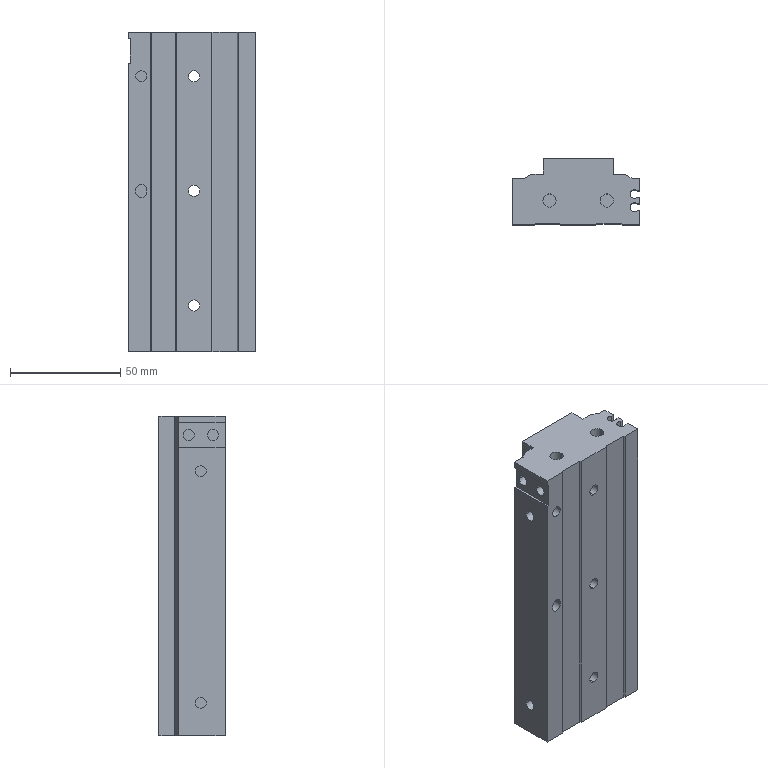Part | NX | 1 solid | 99 faces | box 58 x 30 x 145 mm | volume 176717 mm3 | plane 53 | cylinder 46 | commonest cylinder face diameters 5 x20 5.1 x6 9.5 x6 6 x4 16 x4 17 x4